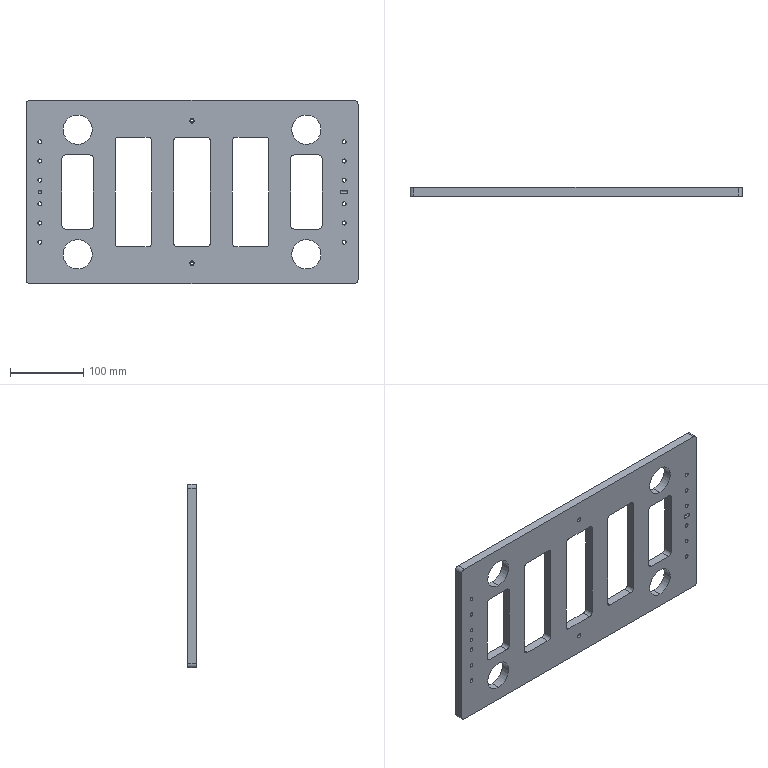Part | SolidWorks | features HoleWzd 5, Fillet 3, ICE 2, Extrusion 1 | 1 solid | 162 faces | box 453 x 12 x 250 mm | volume 916603 mm3 | cylinder 104 | plane 46 | cone 12 | commonest cylinder face diameters 10 x48 5.5 x24 2.5 x8 40 x8 3.4 x4 5 x4